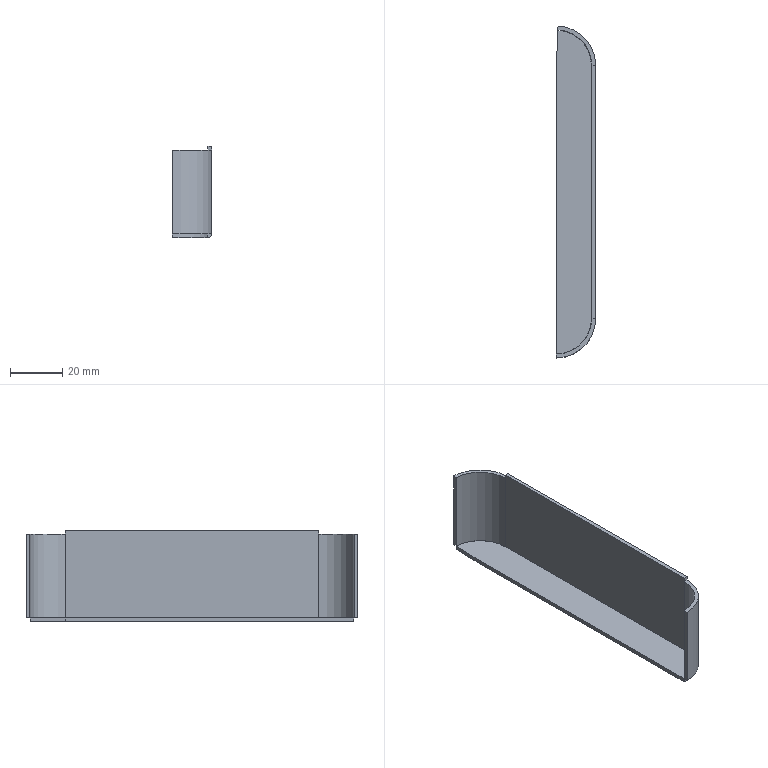Part | SolidWorks | features SMBaseFlange 2, EdgeFlange 1, FlatPattern 1, ICE 1, SheetMetal 1 | 1 solid | 26 faces | box 15 x 126.848 x 35 mm | volume 9537 mm3 | plane 19 | cylinder 7 | commonest cylinder face diameters 26.8 x2 27 x2 30 x2 3 x1
STEP:
#1=CARTESIAN_POINT('',(-15.,-61.931,15.25));
#2=VERTEX_POINT('',#1);
#3=CARTESIAN_POINT('',(-15.,-61.931,-16.75));
#4=VERTEX_POINT('',#3);
#5=CARTESIAN_POINT('',(-15.,-61.931,16.75));
#6=DIRECTION('',(0.,0.,-1.));
#7=VECTOR('',#6,1000.);
#8=LINE('',#5,#7);
#9=EDGE_CURVE('',#2,#4,#8,.T.);
#10=ORIENTED_EDGE('',*,*,#9,.F.);
#11=CARTESIAN_POINT('',(-1.5,-48.431,15.25));
#12=VERTEX_POINT('',#11);
#13=CARTESIAN_POINT('',(-15.,-48.431,15.25));
#14=DIRECTION('',(0.,0.,-1.));
#15=DIRECTION('',(1.,0.,0.));
#16=AXIS2_PLACEMENT_3D('',#13,#14,#15);
#17=CIRCLE('',#16,13.5);
#18=EDGE_CURVE('',#12,#2,#17,.T.);
#19=ORIENTED_EDGE('',*,*,#18,.F.);
#20=CARTESIAN_POINT('',(-1.5,-48.431,-16.75));
#21=VERTEX_POINT('',#20);
#22=CARTESIAN_POINT('',(-1.5,-48.431,16.75));
#23=DIRECTION('',(0.,0.,-1.));
#24=VECTOR('',#23,1000.);
#25=LINE('',#22,#24);
#26=EDGE_CURVE('',#12,#21,#25,.T.);
#27=ORIENTED_EDGE('',*,*,#26,.T.);
#28=CARTESIAN_POINT('',(-15.,-48.431,-16.75));
#29=DIRECTION('',(0.,0.,1.));
#30=DIRECTION('',(1.,0.,0.));
#31=AXIS2_PLACEMENT_3D('',#28,#29,#30);
#32=CIRCLE('',#31,13.5);
#33=EDGE_CURVE('',#4,#21,#32,.T.);
#34=ORIENTED_EDGE('',*,*,#33,.F.);
#35=EDGE_LOOP('',(#10,#19,#27,#34));
#36=FACE_OUTER_BOUND('',#35,.T.);
#37=CARTESIAN_POINT('',(-15.,-48.431,16.75));
#38=DIRECTION('',(0.,0.,-1.));
#39=DIRECTION('',(-1.,0.,0.));
#40=AXIS2_PLACEMENT_3D('',#37,#38,#39);
#41=CYLINDRICAL_SURFACE('',#40,13.5);
#42=ADVANCED_FACE('',(#36),#41,.F.);
#43=CARTESIAN_POINT('',(-15.,-63.431,15.25));
#44=VERTEX_POINT('',#43);
#45=CARTESIAN_POINT('',(-15.,-63.431,-16.75));
#46=VERTEX_POINT('',#45);
#47=CARTESIAN_POINT('',(-15.,-63.431,16.75));
#48=DIRECTION('',(0.,0.,-1.));
#49=VECTOR('',#48,1000.);
#50=LINE('',#47,#49);
#51=EDGE_CURVE('',#44,#46,#50,.T.);
#52=ORIENTED_EDGE('',*,*,#51,.F.);
#53=CARTESIAN_POINT('',(-15.,-63.431,15.25));
#54=DIRECTION('',(0.000000038,-1.,0.));
#55=VECTOR('',#54,1000.);
#56=LINE('',#53,#55);
#57=EDGE_CURVE('',#2,#44,#56,.T.);
#58=ORIENTED_EDGE('',*,*,#57,.F.);
#59=ORIENTED_EDGE('',*,*,#9,.T.);
#60=CARTESIAN_POINT('',(-15.,-63.431,-16.75));
#61=DIRECTION('',(-0.000000038,1.,0.));
#62=VECTOR('',#61,1000.);
#63=LINE('',#60,#62);
#64=EDGE_CURVE('',#46,#4,#63,.T.);
#65=ORIENTED_EDGE('',*,*,#64,.F.);
#66=EDGE_LOOP('',(#52,#58,#59,#65));
#67=FACE_OUTER_BOUND('',#66,.T.);
#68=CARTESIAN_POINT('',(-15.,-63.431,16.75));
#69=DIRECTION('',(-1.,-0.000000038,0.));
#70=DIRECTION('',(0.000000038,-1.,0.));
#71=AXIS2_PLACEMENT_3D('',#68,#69,#70);
#72=PLANE('',#71);
#73=ADVANCED_FACE('',(#67),#72,.T.);
#74=CARTESIAN_POINT('',(0.000001671,-48.431,15.25));
#75=VERTEX_POINT('',#74);
#76=CARTESIAN_POINT('',(-15.,-48.431,15.25));
#77=DIRECTION('',(0.,0.,1.));
#78=DIRECTION('',(1.,0.,0.));
#79=AXIS2_PLACEMENT_3D('',#76,#77,#78);
#80=CIRCLE('',#79,15.);
#81=EDGE_CURVE('',#44,#75,#80,.T.);
#82=ORIENTED_EDGE('',*,*,#81,.F.);
#83=ORIENTED_EDGE('',*,*,#51,.T.);
#84=CARTESIAN_POINT('',(0.000001671,-48.431,-16.75));
#85=VERTEX_POINT('',#84);
#86=CARTESIAN_POINT('',(-15.,-48.431,-16.75));
#87=DIRECTION('',(0.,0.,1.));
#88=DIRECTION('',(1.,0.,0.));
#89=AXIS2_PLACEMENT_3D('',#86,#87,#88);
#90=CIRCLE('',#89,15.);
#91=EDGE_CURVE('',#46,#85,#90,.T.);
#92=ORIENTED_EDGE('',*,*,#91,.T.);
#93=CARTESIAN_POINT('',(0.000001671,-48.431,16.75));
#94=DIRECTION('',(0.,0.,-1.));
#95=VECTOR('',#94,1000.);
#96=LINE('',#93,#95);
#97=EDGE_CURVE('',#75,#85,#96,.T.);
#98=ORIENTED_EDGE('',*,*,#97,.F.);
#99=EDGE_LOOP('',(#82,#83,#92,#98));
#100=FACE_OUTER_BOUND('',#99,.T.);
#101=CARTESIAN_POINT('',(-15.,-48.431,16.75));
#102=DIRECTION('',(0.,0.,-1.));
#103=DIRECTION('',(-1.,0.,0.));
#104=AXIS2_PLACEMENT_3D('',#101,#102,#103);
#105=CYLINDRICAL_SURFACE('',#104,15.);
#106=ADVANCED_FACE('',(#100),#105,.T.);
#107=CARTESIAN_POINT('',(-0.000001671,48.431,15.25));
#108=VERTEX_POINT('',#107);
#109=CARTESIAN_POINT('',(-14.36,63.417,15.25));
#110=VERTEX_POINT('',#109);
#111=CARTESIAN_POINT('',(-15.,48.431,15.25));
#112=DIRECTION('',(0.,0.,1.));
#113=DIRECTION('',(1.,0.,0.));
#114=AXIS2_PLACEMENT_3D('',#111,#112,#113);
#115=CIRCLE('',#114,15.);
#116=EDGE_CURVE('',#108,#110,#115,.T.);
#117=ORIENTED_EDGE('',*,*,#116,.F.);
#118=CARTESIAN_POINT('',(-0.000001671,48.431,-16.75));
#119=VERTEX_POINT('',#118);
#120=CARTESIAN_POINT('',(-0.000001671,48.431,16.75));
#121=DIRECTION('',(0.,0.,-1.));
#122=VECTOR('',#121,1000.);
#123=LINE('',#120,#122);
#124=EDGE_CURVE('',#108,#119,#123,.T.);
#125=ORIENTED_EDGE('',*,*,#124,.T.);
#126=CARTESIAN_POINT('',(-14.36,63.417,-16.75));
#127=VERTEX_POINT('',#126);
#128=CARTESIAN_POINT('',(-15.,48.431,-16.75));
#129=DIRECTION('',(0.,0.,1.));
#130=DIRECTION('',(1.,0.,0.));
#131=AXIS2_PLACEMENT_3D('',#128,#129,#130);
#132=CIRCLE('',#131,15.);
#133=EDGE_CURVE('',#119,#127,#132,.T.);
#134=ORIENTED_EDGE('',*,*,#133,.T.);
#135=CARTESIAN_POINT('',(-14.36,63.417,16.75));
#136=DIRECTION('',(0.,0.,-1.));
#137=VECTOR('',#136,1000.);
#138=LINE('',#135,#137);
#139=EDGE_CURVE('',#110,#127,#138,.T.);
#140=ORIENTED_EDGE('',*,*,#139,.F.);
#141=EDGE_LOOP('',(#117,#125,#134,#140));
#142=FACE_OUTER_BOUND('',#141,.T.);
#143=CARTESIAN_POINT('',(-15.,48.431,16.75));
#144=DIRECTION('',(0.,0.,-1.));
#145=DIRECTION('',(-1.,0.,0.));
#146=AXIS2_PLACEMENT_3D('',#143,#144,#145);
#147=CYLINDRICAL_SURFACE('',#146,15.);
#148=ADVANCED_FACE('',(#142),#147,.T.);
#149=CARTESIAN_POINT('',(-14.424,61.919,15.25));
#150=VERTEX_POINT('',#149);
#151=CARTESIAN_POINT('',(-14.424,61.919,-16.75));
#152=VERTEX_POINT('',#151);
#153=CARTESIAN_POINT('',(-14.424,61.919,16.75));
#154=DIRECTION('',(0.,0.,-1.));
#155=VECTOR('',#154,1000.);
#156=LINE('',#153,#155);
#157=EDGE_CURVE('',#150,#152,#156,.T.);
#158=ORIENTED_EDGE('',*,*,#157,.F.);
#159=CARTESIAN_POINT('',(-14.424,61.919,15.25));
#160=DIRECTION('',(-0.04269,-0.9991,0.));
#161=VECTOR('',#160,1000.);
#162=LINE('',#159,#161);
#163=EDGE_CURVE('',#110,#150,#162,.T.);
#164=ORIENTED_EDGE('',*,*,#163,.F.);
#165=ORIENTED_EDGE('',*,*,#139,.T.);
#166=CARTESIAN_POINT('',(-14.424,61.919,-16.75));
#167=DIRECTION('',(0.04269,0.9991,0.));
#168=VECTOR('',#167,1000.);
#169=LINE('',#166,#168);
#170=EDGE_CURVE('',#152,#127,#169,.T.);
#171=ORIENTED_EDGE('',*,*,#170,.F.);
#172=EDGE_LOOP('',(#158,#164,#165,#171));
#173=FACE_OUTER_BOUND('',#172,.T.);
#174=CARTESIAN_POINT('',(-14.424,61.919,16.75));
#175=DIRECTION('',(-0.9991,0.04269,0.));
#176=DIRECTION('',(-0.04269,-0.9991,0.));
#177=AXIS2_PLACEMENT_3D('',#174,#175,#176);
#178=PLANE('',#177);
#179=ADVANCED_FACE('',(#173),#178,.T.);
#180=CARTESIAN_POINT('',(-1.5,48.431,15.25));
#181=VERTEX_POINT('',#180);
#182=CARTESIAN_POINT('',(-1.5,48.431,-16.75));
#183=VERTEX_POINT('',#182);
#184=CARTESIAN_POINT('',(-1.5,48.431,16.75));
#185=DIRECTION('',(0.,0.,-1.));
#186=VECTOR('',#185,1000.);
#187=LINE('',#184,#186);
#188=EDGE_CURVE('',#181,#183,#187,.T.);
#189=ORIENTED_EDGE('',*,*,#188,.F.);
#190=CARTESIAN_POINT('',(-15.,48.431,15.25));
#191=DIRECTION('',(0.,0.,-1.));
#192=DIRECTION('',(1.,0.,0.));
#193=AXIS2_PLACEMENT_3D('',#190,#191,#192);
#194=CIRCLE('',#193,13.5);
#195=EDGE_CURVE('',#150,#181,#194,.T.);
#196=ORIENTED_EDGE('',*,*,#195,.F.);
#197=ORIENTED_EDGE('',*,*,#157,.T.);
#198=CARTESIAN_POINT('',(-15.,48.431,-16.75));
#199=DIRECTION('',(0.,0.,1.));
#200=DIRECTION('',(1.,0.,0.));
#201=AXIS2_PLACEMENT_3D('',#198,#199,#200);
#202=CIRCLE('',#201,13.5);
#203=EDGE_CURVE('',#183,#152,#202,.T.);
#204=ORIENTED_EDGE('',*,*,#203,.F.);
#205=EDGE_LOOP('',(#189,#196,#197,#204));
#206=FACE_OUTER_BOUND('',#205,.T.);
#207=CARTESIAN_POINT('',(-15.,48.431,16.75));
#208=DIRECTION('',(0.,0.,-1.));
#209=DIRECTION('',(-1.,0.,0.));
#210=AXIS2_PLACEMENT_3D('',#207,#208,#209);
#211=CYLINDRICAL_SURFACE('',#210,13.5);
#212=ADVANCED_FACE('',(#206),#211,.F.);
#213=CARTESIAN_POINT('',(0.000001671,-48.431,-16.75));
#214=DIRECTION('',(-1.,-0.000000034,0.));
#215=VECTOR('',#214,1000.);
#216=LINE('',#213,#215);
#217=EDGE_CURVE('',#85,#21,#216,.T.);
#218=ORIENTED_EDGE('',*,*,#217,.F.);
#219=ORIENTED_EDGE('',*,*,#91,.F.);
#220=ORIENTED_EDGE('',*,*,#64,.T.);
#221=ORIENTED_EDGE('',*,*,#33,.T.);
#222=EDGE_LOOP('',(#218,#219,#220,#221));
#223=FACE_OUTER_BOUND('',#222,.T.);
#224=CARTESIAN_POINT('',(0.000001671,-48.431,-16.75));
#225=DIRECTION('',(0.,0.,-1.));
#226=DIRECTION('',(-1.,0.,0.));
#227=AXIS2_PLACEMENT_3D('',#224,#225,#226);
#228=PLANE('',#227);
#229=ADVANCED_FACE('',(#223),#228,.T.);
#230=CARTESIAN_POINT('',(-1.5,48.431,-16.75));
#231=DIRECTION('',(1.,0.000000034,0.));
#232=VECTOR('',#231,1000.);
#233=LINE('',#230,#232);
#234=EDGE_CURVE('',#183,#119,#233,.T.);
#235=ORIENTED_EDGE('',*,*,#234,.F.);
#236=ORIENTED_EDGE('',*,*,#203,.T.);
#237=ORIENTED_EDGE('',*,*,#170,.T.);
#238=ORIENTED_EDGE('',*,*,#133,.F.);
#239=EDGE_LOOP('',(#235,#236,#237,#238));
#240=FACE_OUTER_BOUND('',#239,.T.);
#241=CARTESIAN_POINT('',(-1.5,48.431,-16.75));
#242=DIRECTION('',(0.,0.,-1.));
#243=DIRECTION('',(-1.,0.,0.));
#244=AXIS2_PLACEMENT_3D('',#241,#242,#243);
#245=PLANE('',#244);
#246=ADVANCED_FACE('',(#240),#245,.T.);
#247=CARTESIAN_POINT('',(-1.5,48.431,-16.75));
#248=DIRECTION('',(-0.000000034,1.,0.));
#249=VECTOR('',#248,1000.);
#250=LINE('',#247,#249);
#251=EDGE_CURVE('',#21,#183,#250,.T.);
#252=ORIENTED_EDGE('',*,*,#251,.F.);
#253=ORIENTED_EDGE('',*,*,#26,.F.);
#254=CARTESIAN_POINT('',(-1.5,-48.431,16.75));
#255=VERTEX_POINT('',#254);
#256=CARTESIAN_POINT('',(-1.5,-48.431,16.75));
#257=DIRECTION('',(0.,0.,-1.));
#258=VECTOR('',#257,1000.);
#259=LINE('',#256,#258);
#260=EDGE_CURVE('',#255,#12,#259,.T.);
#261=ORIENTED_EDGE('',*,*,#260,.F.);
#262=CARTESIAN_POINT('',(-1.5,48.431,16.75));
#263=VERTEX_POINT('',#262);
#264=CARTESIAN_POINT('',(-1.5,48.431,16.75));
#265=DIRECTION('',(-0.000000034,1.,0.));
#266=VECTOR('',#265,1000.);
#267=LINE('',#264,#266);
#268=EDGE_CURVE('',#255,#263,#267,.T.);
#269=ORIENTED_EDGE('',*,*,#268,.T.);
#270=CARTESIAN_POINT('',(-1.5,48.431,16.75));
#271=DIRECTION('',(0.,0.,-1.));
#272=VECTOR('',#271,1000.);
#273=LINE('',#270,#272);
#274=EDGE_CURVE('',#263,#181,#273,.T.);
#275=ORIENTED_EDGE('',*,*,#274,.T.);
#276=ORIENTED_EDGE('',*,*,#188,.T.);
#277=EDGE_LOOP('',(#252,#253,#261,#269,#275,#276));
#278=FACE_OUTER_BOUND('',#277,.T.);
#279=CARTESIAN_POINT('',(-1.5,48.431,16.75));
#280=DIRECTION('',(-1.,-0.000000034,0.));
#281=DIRECTION('',(0.000000034,-1.,0.));
#282=AXIS2_PLACEMENT_3D('',#279,#280,#281);
#283=PLANE('',#282);
#284=ADVANCED_FACE('',(#278),#283,.T.);
#285=CARTESIAN_POINT('',(-0.000001671,48.431,-16.75));
#286=DIRECTION('',(-0.000000034,1.,0.));
#287=VECTOR('',#286,1000.);
#288=LINE('',#285,#287);
#289=EDGE_CURVE('',#85,#119,#288,.T.);
#290=ORIENTED_EDGE('',*,*,#289,.T.);
#291=ORIENTED_EDGE('',*,*,#124,.F.);
#292=CARTESIAN_POINT('',(-0.000001671,48.431,16.75));
#293=VERTEX_POINT('',#292);
#294=CARTESIAN_POINT('',(-0.000001671,48.431,16.75));
#295=DIRECTION('',(0.,0.,-1.));
#296=VECTOR('',#295,1000.);
#297=LINE('',#294,#296);
#298=EDGE_CURVE('',#293,#108,#297,.T.);
#299=ORIENTED_EDGE('',*,*,#298,.F.);
#300=CARTESIAN_POINT('',(0.000001671,-48.431,16.75));
#301=VERTEX_POINT('',#300);
#302=CARTESIAN_POINT('',(-0.000001671,48.431,16.75));
#303=DIRECTION('',(-0.000000034,1.,0.));
#304=VECTOR('',#303,1000.);
#305=LINE('',#302,#304);
#306=EDGE_CURVE('',#301,#293,#305,.T.);
#307=ORIENTED_EDGE('',*,*,#306,.F.);
#308=CARTESIAN_POINT('',(0.000001671,-48.431,16.75));
#309=DIRECTION('',(0.,0.,-1.));
#310=VECTOR('',#309,1000.);
#311=LINE('',#308,#310);
#312=EDGE_CURVE('',#301,#75,#311,.T.);
#313=ORIENTED_EDGE('',*,*,#312,.T.);
#314=ORIENTED_EDGE('',*,*,#97,.T.);
#315=EDGE_LOOP('',(#290,#291,#299,#307,#313,#314));
#316=FACE_OUTER_BOUND('',#315,.T.);
#317=CARTESIAN_POINT('',(-0.000001671,48.431,16.75));
#318=DIRECTION('',(-1.,-0.000000034,0.));
#319=DIRECTION('',(0.000000034,-1.,0.));
#320=AXIS2_PLACEMENT_3D('',#317,#318,#319);
#321=PLANE('',#320);
#322=ADVANCED_FACE('',(#316),#321,.F.);
#323=ORIENTED_EDGE('',*,*,#306,.T.);
#324=CARTESIAN_POINT('',(-0.000001671,48.431,16.75));
#325=DIRECTION('',(-1.,-0.000000034,0.));
#326=VECTOR('',#325,1000.);
#327=LINE('',#324,#326);
#328=EDGE_CURVE('',#293,#263,#327,.T.);
#329=ORIENTED_EDGE('',*,*,#328,.T.);
#330=ORIENTED_EDGE('',*,*,#268,.F.);
#331=CARTESIAN_POINT('',(-1.5,-48.431,16.75));
#332=DIRECTION('',(1.,0.000000034,0.));
#333=VECTOR('',#332,1000.);
#334=LINE('',#331,#333);
#335=EDGE_CURVE('',#255,#301,#334,.T.);
#336=ORIENTED_EDGE('',*,*,#335,.T.);
#337=EDGE_LOOP('',(#323,#329,#330,#336));
#338=FACE_OUTER_BOUND('',#337,.T.);
#339=CARTESIAN_POINT('',(-15.,48.431,16.75));
#340=DIRECTION('',(0.,0.,1.));
#341=DIRECTION('',(1.,0.,0.));
#342=AXIS2_PLACEMENT_3D('',#339,#340,#341);
#343=PLANE('',#342);
#344=ADVANCED_FACE('',(#338),#343,.T.);
#345=CARTESIAN_POINT('',(-1.5,-48.431,-18.25));
#346=VERTEX_POINT('',#345);
#347=CARTESIAN_POINT('',(-1.5,-48.431,-16.75));
#348=DIRECTION('',(-0.000000034,1.,0.));
#349=DIRECTION('',(-1.,-0.000000034,0.));
#350=AXIS2_PLACEMENT_3D('',#347,#348,#349);
#351=CIRCLE('',#350,1.5);
#352=EDGE_CURVE('',#85,#346,#351,.T.);
#353=ORIENTED_EDGE('',*,*,#352,.F.);
#354=ORIENTED_EDGE('',*,*,#217,.T.);
#355=CARTESIAN_POINT('',(-1.5,-48.431,-18.25));
#356=DIRECTION('',(0.,0.,1.));
#357=VECTOR('',#356,1000.);
#358=LINE('',#355,#357);
#359=EDGE_CURVE('',#346,#21,#358,.T.);
#360=ORIENTED_EDGE('',*,*,#359,.F.);
#361=EDGE_LOOP('',(#353,#354,#360));
#362=FACE_OUTER_BOUND('',#361,.T.);
#363=CARTESIAN_POINT('',(0.000001671,-48.431,-16.75));
#364=DIRECTION('',(0.000000034,-1.,0.));
#365=DIRECTION('',(1.,0.000000034,0.));
#366=AXIS2_PLACEMENT_3D('',#363,#364,#365);
#367=PLANE('',#366);
#368=ADVANCED_FACE('',(#362),#367,.T.);
#369=CARTESIAN_POINT('',(-1.5,48.431,-18.25));
#370=VERTEX_POINT('',#369);
#371=CARTESIAN_POINT('',(-1.5,48.431,-16.75));
#372=DIRECTION('',(-0.000000034,1.,0.));
#373=DIRECTION('',(-1.,-0.000000034,0.));
#374=AXIS2_PLACEMENT_3D('',#371,#372,#373);
#375=CIRCLE('',#374,1.5);
#376=EDGE_CURVE('',#119,#370,#375,.T.);
#377=ORIENTED_EDGE('',*,*,#376,.F.);
#378=ORIENTED_EDGE('',*,*,#289,.F.);
#379=ORIENTED_EDGE('',*,*,#352,.T.);
#380=CARTESIAN_POINT('',(-1.5,48.431,-18.25));
#381=DIRECTION('',(-0.000000034,1.,0.));
#382=VECTOR('',#381,1000.);
#383=LINE('',#380,#382);
#384=EDGE_CURVE('',#346,#370,#383,.T.);
#385=ORIENTED_EDGE('',*,*,#384,.T.);
#386=EDGE_LOOP('',(#377,#378,#379,#385));
#387=FACE_OUTER_BOUND('',#386,.T.);
#388=CARTESIAN_POINT('',(-1.5,48.431,-16.75));
#389=DIRECTION('',(-0.000000034,1.,0.));
#390=DIRECTION('',(-1.,-0.000000034,0.));
#391=AXIS2_PLACEMENT_3D('',#388,#389,#390);
#392=CYLINDRICAL_SURFACE('',#391,1.5);
#393=ADVANCED_FACE('',(#387),#392,.T.);
#394=ORIENTED_EDGE('',*,*,#234,.T.);
#395=ORIENTED_EDGE('',*,*,#376,.T.);
#396=CARTESIAN_POINT('',(-1.5,48.431,-18.25));
#397=DIRECTION('',(0.,0.,1.));
#398=VECTOR('',#397,1000.);
#399=LINE('',#396,#398);
#400=EDGE_CURVE('',#370,#183,#399,.T.);
#401=ORIENTED_EDGE('',*,*,#400,.T.);
#402=EDGE_LOOP('',(#394,#395,#401));
#403=FACE_OUTER_BOUND('',#402,.T.);
#404=CARTESIAN_POINT('',(-0.000001671,48.431,-16.75));
#405=DIRECTION('',(0.000000034,-1.,0.));
#406=DIRECTION('',(1.,0.000000034,0.));
#407=AXIS2_PLACEMENT_3D('',#404,#405,#406);
#408=PLANE('',#407);
#409=ADVANCED_FACE('',(#403),#408,.F.);
#410=CARTESIAN_POINT('',(-1.6,-48.431,-16.75));
#411=VERTEX_POINT('',#410);
#412=CARTESIAN_POINT('',(-1.6,-48.431,-18.25));
#413=VERTEX_POINT('',#412);
#414=CARTESIAN_POINT('',(-1.6,-48.431,-16.75));
#415=DIRECTION('',(0.,0.,-1.));
#416=VECTOR('',#415,1000.);
#417=LINE('',#414,#416);
#418=EDGE_CURVE('',#411,#413,#417,.T.);
#419=ORIENTED_EDGE('',*,*,#418,.T.);
#420=CARTESIAN_POINT('',(-1.5,-48.431,-18.25));
#421=DIRECTION('',(1.,0.000000034,0.));
#422=VECTOR('',#421,1000.);
#423=LINE('',#420,#422);
#424=EDGE_CURVE('',#413,#346,#423,.T.);
#425=ORIENTED_EDGE('',*,*,#424,.T.);
#426=ORIENTED_EDGE('',*,*,#359,.T.);
#427=CARTESIAN_POINT('',(-1.5,-48.431,-16.75));
#428=DIRECTION('',(1.,0.000000034,0.));
#429=VECTOR('',#428,1000.);
#430=LINE('',#427,#429);
#431=EDGE_CURVE('',#411,#21,#430,.T.);
#432=ORIENTED_EDGE('',*,*,#431,.F.);
#433=EDGE_LOOP('',(#419,#425,#426,#432));
#434=FACE_OUTER_BOUND('',#433,.T.);
#435=CARTESIAN_POINT('',(-1.5,-48.431,-18.25));
#436=DIRECTION('',(0.000000034,-1.,0.));
#437=DIRECTION('',(1.,0.000000034,0.));
#438=AXIS2_PLACEMENT_3D('',#435,#436,#437);
#439=PLANE('',#438);
#440=ADVANCED_FACE('',(#434),#439,.T.);
#441=CARTESIAN_POINT('',(-15.,48.431,-16.75));
#442=VERTEX_POINT('',#441);
#443=CARTESIAN_POINT('',(-15.,-48.431,-16.75));
#444=VERTEX_POINT('',#443);
#445=CARTESIAN_POINT('',(-15.,-48.431,-16.75));
#446=DIRECTION('',(0.000000034,-1.,0.));
#447=VECTOR('',#446,1000.);
#448=LINE('',#445,#447);
#449=EDGE_CURVE('',#442,#444,#448,.T.);
#450=ORIENTED_EDGE('',*,*,#449,.F.);
#451=CARTESIAN_POINT('',(-15.,48.431,-18.25));
#452=VERTEX_POINT('',#451);
#453=CARTESIAN_POINT('',(-15.,48.431,-18.25));
#454=DIRECTION('',(0.,0.,1.));
#455=VECTOR('',#454,1000.);
#456=LINE('',#453,#455);
#457=EDGE_CURVE('',#452,#442,#456,.T.);
#458=ORIENTED_EDGE('',*,*,#457,.F.);
#459=CARTESIAN_POINT('',(-15.,-48.431,-18.25));
#460=VERTEX_POINT('',#459);
#461=CARTESIAN_POINT('',(-15.,-48.431,-18.25));
#462=DIRECTION('',(0.000000034,-1.,0.));
#463=VECTOR('',#462,1000.);
#464=LINE('',#461,#463);
#465=EDGE_CURVE('',#452,#460,#464,.T.);
#466=ORIENTED_EDGE('',*,*,#465,.T.);
#467=CARTESIAN_POINT('',(-15.,-61.831,-18.25));
#468=VERTEX_POINT('',#467);
#469=CARTESIAN_POINT('',(-15.,-61.831,-18.25));
#470=DIRECTION('',(0.,1.,0.));
#471=VECTOR('',#470,1000.);
#472=LINE('',#469,#471);
#473=EDGE_CURVE('',#468,#460,#472,.T.);
#474=ORIENTED_EDGE('',*,*,#473,.F.);
#475=CARTESIAN_POINT('',(-15.,-61.831,-16.75));
#476=VERTEX_POINT('',#475);
#477=CARTESIAN_POINT('',(-15.,-61.831,-16.75));
#478=DIRECTION('',(0.,0.,-1.));
#479=VECTOR('',#478,1000.);
#480=LINE('',#477,#479);
#481=EDGE_CURVE('',#476,#468,#480,.T.);
#482=ORIENTED_EDGE('',*,*,#481,.F.);
#483=CARTESIAN_POINT('',(-15.,-61.831,-16.75));
#484=DIRECTION('',(0.,1.,0.));
#485=VECTOR('',#484,1000.);
#486=LINE('',#483,#485);
#487=EDGE_CURVE('',#476,#444,#486,.T.);
#488=ORIENTED_EDGE('',*,*,#487,.T.);
#489=EDGE_LOOP('',(#450,#458,#466,#474,#482,#488));
#490=FACE_OUTER_BOUND('',#489,.T.);
#491=CARTESIAN_POINT('',(-15.,-48.431,-18.25));
#492=DIRECTION('',(-1.,-0.000000034,0.));
#493=DIRECTION('',(0.000000034,-1.,0.));
#494=AXIS2_PLACEMENT_3D('',#491,#492,#493);
#495=PLANE('',#494);
#496=ADVANCED_FACE('',(#490),#495,.T.);
#497=CARTESIAN_POINT('',(-1.6,48.431,-16.75));
#498=VERTEX_POINT('',#497);
#499=CARTESIAN_POINT('',(-1.6,48.431,-18.25));
#500=VERTEX_POINT('',#499);
#501=CARTESIAN_POINT('',(-1.6,48.431,-16.75));
#502=DIRECTION('',(0.,0.,-1.));
#503=VECTOR('',#502,1000.);
#504=LINE('',#501,#503);
#505=EDGE_CURVE('',#498,#500,#504,.T.);
#506=ORIENTED_EDGE('',*,*,#505,.F.);
#507=CARTESIAN_POINT('',(-15.,48.431,-16.75));
#508=DIRECTION('',(-1.,-0.000000034,0.));
#509=VECTOR('',#508,1000.);
#510=LINE('',#507,#509);
#511=EDGE_CURVE('',#183,#498,#510,.T.);
#512=ORIENTED_EDGE('',*,*,#511,.F.);
#513=ORIENTED_EDGE('',*,*,#400,.F.);
#514=CARTESIAN_POINT('',(-15.,48.431,-18.25));
#515=DIRECTION('',(-1.,-0.000000034,0.));
#516=VECTOR('',#515,1000.);
#517=LINE('',#514,#516);
#518=EDGE_CURVE('',#370,#500,#517,.T.);
#519=ORIENTED_EDGE('',*,*,#518,.T.);
#520=EDGE_LOOP('',(#506,#512,#513,#519));
#521=FACE_OUTER_BOUND('',#520,.T.);
#522=CARTESIAN_POINT('',(-15.,48.431,-18.25));
#523=DIRECTION('',(-0.000000034,1.,0.));
#524=DIRECTION('',(-1.,-0.000000034,0.));
#525=AXIS2_PLACEMENT_3D('',#522,#523,#524);
#526=PLANE('',#525);
#527=ADVANCED_FACE('',(#521),#526,.T.);
#528=ORIENTED_EDGE('',*,*,#384,.F.);
#529=ORIENTED_EDGE('',*,*,#424,.F.);
#530=CARTESIAN_POINT('',(-15.,-48.431,-18.25));
#531=DIRECTION('',(0.,0.,-1.));
#532=DIRECTION('',(-1.,0.,0.));
#533=AXIS2_PLACEMENT_3D('',#530,#531,#532);
#534=CIRCLE('',#533,13.4);
#535=EDGE_CURVE('',#413,#468,#534,.T.);
#536=ORIENTED_EDGE('',*,*,#535,.T.);
#537=ORIENTED_EDGE('',*,*,#473,.T.);
#538=ORIENTED_EDGE('',*,*,#465,.F.);
#539=CARTESIAN_POINT('',(-14.428,61.819,-18.25));
#540=VERTEX_POINT('',#539);
#541=CARTESIAN_POINT('',(-15.,48.431,-18.25));
#542=DIRECTION('',(0.04269,0.9991,0.));
#543=VECTOR('',#542,1000.);
#544=LINE('',#541,#543);
#545=EDGE_CURVE('',#452,#540,#544,.T.);
#546=ORIENTED_EDGE('',*,*,#545,.T.);
#547=CARTESIAN_POINT('',(-15.,48.431,-18.25));
#548=DIRECTION('',(0.,0.,-1.));
#549=DIRECTION('',(-1.,0.,0.));
#550=AXIS2_PLACEMENT_3D('',#547,#548,#549);
#551=CIRCLE('',#550,13.4);
#552=EDGE_CURVE('',#540,#500,#551,.T.);
#553=ORIENTED_EDGE('',*,*,#552,.T.);
#554=ORIENTED_EDGE('',*,*,#518,.F.);
#555=EDGE_LOOP('',(#528,#529,#536,#537,#538,#546,#553,#554));
#556=FACE_OUTER_BOUND('',#555,.T.);
#557=CARTESIAN_POINT('',(-1.5,-48.431,-18.25));
#558=DIRECTION('',(0.,0.,-1.));
#559=DIRECTION('',(-1.,0.,0.));
#560=AXIS2_PLACEMENT_3D('',#557,#558,#559);
#561=PLANE('',#560);
#562=ADVANCED_FACE('',(#556),#561,.T.);
#563=ORIENTED_EDGE('',*,*,#251,.T.);
#564=ORIENTED_EDGE('',*,*,#511,.T.);
#565=CARTESIAN_POINT('',(-14.428,61.819,-16.75));
#566=VERTEX_POINT('',#565);
#567=CARTESIAN_POINT('',(-15.,48.431,-16.75));
#568=DIRECTION('',(0.,0.,-1.));
#569=DIRECTION('',(-1.,0.,0.));
#570=AXIS2_PLACEMENT_3D('',#567,#568,#569);
#571=CIRCLE('',#570,13.4);
#572=EDGE_CURVE('',#566,#498,#571,.T.);
#573=ORIENTED_EDGE('',*,*,#572,.F.);
#574=CARTESIAN_POINT('',(-15.,48.431,-16.75));
#575=DIRECTION('',(0.04269,0.9991,0.));
#576=VECTOR('',#575,1000.);
#577=LINE('',#574,#576);
#578=EDGE_CURVE('',#442,#566,#577,.T.);
#579=ORIENTED_EDGE('',*,*,#578,.F.);
#580=ORIENTED_EDGE('',*,*,#449,.T.);
#581=ORIENTED_EDGE('',*,*,#487,.F.);
#582=CARTESIAN_POINT('',(-15.,-48.431,-16.75));
#583=DIRECTION('',(0.,0.,-1.));
#584=DIRECTION('',(-1.,0.,0.));
#585=AXIS2_PLACEMENT_3D('',#582,#583,#584);
#586=CIRCLE('',#585,13.4);
#587=EDGE_CURVE('',#411,#476,#586,.T.);
#588=ORIENTED_EDGE('',*,*,#587,.F.);
#589=ORIENTED_EDGE('',*,*,#431,.T.);
#590=EDGE_LOOP('',(#563,#564,#573,#579,#580,#581,#588,#589));
#591=FACE_OUTER_BOUND('',#590,.T.);
#592=CARTESIAN_POINT('',(-1.5,-48.431,-16.75));
#593=DIRECTION('',(0.,0.,-1.));
#594=DIRECTION('',(-1.,0.,0.));
#595=AXIS2_PLACEMENT_3D('',#592,#593,#594);
#596=PLANE('',#595);
#597=ADVANCED_FACE('',(#591),#596,.F.);
#598=ORIENTED_EDGE('',*,*,#545,.F.);
#599=ORIENTED_EDGE('',*,*,#457,.T.);
#600=ORIENTED_EDGE('',*,*,#578,.T.);
#601=CARTESIAN_POINT('',(-14.428,61.819,-16.75));
#602=DIRECTION('',(0.,0.,-1.));
#603=VECTOR('',#602,1000.);
#604=LINE('',#601,#603);
#605=EDGE_CURVE('',#566,#540,#604,.T.);
#606=ORIENTED_EDGE('',*,*,#605,.T.);
#607=EDGE_LOOP('',(#598,#599,#600,#606));
#608=FACE_OUTER_BOUND('',#607,.T.);
#609=CARTESIAN_POINT('',(-15.,48.431,-16.75));
#610=DIRECTION('',(-0.9991,0.04269,0.));
#611=DIRECTION('',(-0.04269,-0.9991,0.));
#612=AXIS2_PLACEMENT_3D('',#609,#610,#611);
#613=PLANE('',#612);
#614=ADVANCED_FACE('',(#608),#613,.T.);
#615=ORIENTED_EDGE('',*,*,#552,.F.);
#616=ORIENTED_EDGE('',*,*,#605,.F.);
#617=ORIENTED_EDGE('',*,*,#572,.T.);
#618=ORIENTED_EDGE('',*,*,#505,.T.);
#619=EDGE_LOOP('',(#615,#616,#617,#618));
#620=FACE_OUTER_BOUND('',#619,.T.);
#621=CARTESIAN_POINT('',(-15.,48.431,-16.75));
#622=DIRECTION('',(0.,0.,-1.));
#623=DIRECTION('',(-1.,0.,0.));
#624=AXIS2_PLACEMENT_3D('',#621,#622,#623);
#625=CYLINDRICAL_SURFACE('',#624,13.4);
#626=ADVANCED_FACE('',(#620),#625,.T.);
#627=ORIENTED_EDGE('',*,*,#535,.F.);
#628=ORIENTED_EDGE('',*,*,#418,.F.);
#629=ORIENTED_EDGE('',*,*,#587,.T.);
#630=ORIENTED_EDGE('',*,*,#481,.T.);
#631=EDGE_LOOP('',(#627,#628,#629,#630));
#632=FACE_OUTER_BOUND('',#631,.T.);
#633=CARTESIAN_POINT('',(-15.,-48.431,-16.75));
#634=DIRECTION('',(0.,0.,-1.));
#635=DIRECTION('',(-1.,0.,0.));
#636=AXIS2_PLACEMENT_3D('',#633,#634,#635);
#637=CYLINDRICAL_SURFACE('',#636,13.4);
#638=ADVANCED_FACE('',(#632),#637,.T.);
#639=ORIENTED_EDGE('',*,*,#328,.F.);
#640=ORIENTED_EDGE('',*,*,#298,.T.);
#641=CARTESIAN_POINT('',(-0.000001671,48.431,15.25));
#642=DIRECTION('',(1.,0.000000034,0.));
#643=VECTOR('',#642,1000.);
#644=LINE('',#641,#643);
#645=EDGE_CURVE('',#181,#108,#644,.T.);
#646=ORIENTED_EDGE('',*,*,#645,.F.);
#647=ORIENTED_EDGE('',*,*,#274,.F.);
#648=EDGE_LOOP('',(#639,#640,#646,#647));
#649=FACE_OUTER_BOUND('',#648,.T.);
#650=CARTESIAN_POINT('',(-0.000001671,48.431,15.25));
#651=DIRECTION('',(0.000000034,-1.,0.));
#652=DIRECTION('',(1.,0.000000034,0.));
#653=AXIS2_PLACEMENT_3D('',#650,#651,#652);
#654=PLANE('',#653);
#655=ADVANCED_FACE('',(#649),#654,.F.);
#656=ORIENTED_EDGE('',*,*,#116,.T.);
#657=ORIENTED_EDGE('',*,*,#163,.T.);
#658=ORIENTED_EDGE('',*,*,#195,.T.);
#659=ORIENTED_EDGE('',*,*,#645,.T.);
#660=EDGE_LOOP('',(#656,#657,#658,#659));
#661=FACE_OUTER_BOUND('',#660,.T.);
#662=CARTESIAN_POINT('',(-15.,48.431,15.25));
#663=DIRECTION('',(0.,0.,1.));
#664=DIRECTION('',(1.,0.,0.));
#665=AXIS2_PLACEMENT_3D('',#662,#663,#664);
#666=PLANE('',#665);
#667=ADVANCED_FACE('',(#661),#666,.T.);
#668=ORIENTED_EDGE('',*,*,#335,.F.);
#669=ORIENTED_EDGE('',*,*,#260,.T.);
#670=CARTESIAN_POINT('',(-1.5,-48.431,15.25));
#671=DIRECTION('',(-1.,-0.000000034,0.));
#672=VECTOR('',#671,1000.);
#673=LINE('',#670,#672);
#674=EDGE_CURVE('',#75,#12,#673,.T.);
#675=ORIENTED_EDGE('',*,*,#674,.F.);
#676=ORIENTED_EDGE('',*,*,#312,.F.);
#677=EDGE_LOOP('',(#668,#669,#675,#676));
#678=FACE_OUTER_BOUND('',#677,.T.);
#679=CARTESIAN_POINT('',(-1.5,-48.431,15.25));
#680=DIRECTION('',(-0.000000034,1.,0.));
#681=DIRECTION('',(-1.,-0.000000034,0.));
#682=AXIS2_PLACEMENT_3D('',#679,#680,#681);
#683=PLANE('',#682);
#684=ADVANCED_FACE('',(#678),#683,.F.);
#685=ORIENTED_EDGE('',*,*,#81,.T.);
#686=ORIENTED_EDGE('',*,*,#674,.T.);
#687=ORIENTED_EDGE('',*,*,#18,.T.);
#688=ORIENTED_EDGE('',*,*,#57,.T.);
#689=EDGE_LOOP('',(#685,#686,#687,#688));
#690=FACE_OUTER_BOUND('',#689,.T.);
#691=CARTESIAN_POINT('',(-15.,-48.431,15.25));
#692=DIRECTION('',(0.,0.,1.));
#693=DIRECTION('',(1.,0.,0.));
#694=AXIS2_PLACEMENT_3D('',#691,#692,#693);
#695=PLANE('',#694);
#696=ADVANCED_FACE('',(#690),#695,.T.);
#697=CLOSED_SHELL('',(#42,#73,#106,#148,#179,#212,#229,#246,#284,#322,#344,#368,#393,#409,#440,#496,#527,#562,#597,#614,#626,#638,#655,#667,#684,#696));
#698=MANIFOLD_SOLID_BREP('',#697);
#699=CARTESIAN_POINT('',(0.,0.,0.));
#700=DIRECTION('',(0.,0.,1.));
#701=DIRECTION('',(1.,0.,0.));
#702=AXIS2_PLACEMENT_3D('',#699,#700,#701);
#703=(LENGTH_UNIT()NAMED_UNIT(*)SI_UNIT(.MILLI.,.METRE.));
#704=UNCERTAINTY_MEASURE_WITH_UNIT(LENGTH_MEASURE(0.00001),#703,'','');
#705=(NAMED_UNIT(*)PLANE_ANGLE_UNIT()SI_UNIT($,.RADIAN.));
#706=(NAMED_UNIT(*)SI_UNIT($,.STERADIAN.)SOLID_ANGLE_UNIT());
#707=(GEOMETRIC_REPRESENTATION_CONTEXT(3)GLOBAL_UNCERTAINTY_ASSIGNED_CONTEXT((#704))GLOBAL_UNIT_ASSIGNED_CONTEXT((#703,#705,#706))REPRESENTATION_CONTEXT('',''));
#708=ADVANCED_BREP_SHAPE_REPRESENTATION('',(#698,#702),#707);